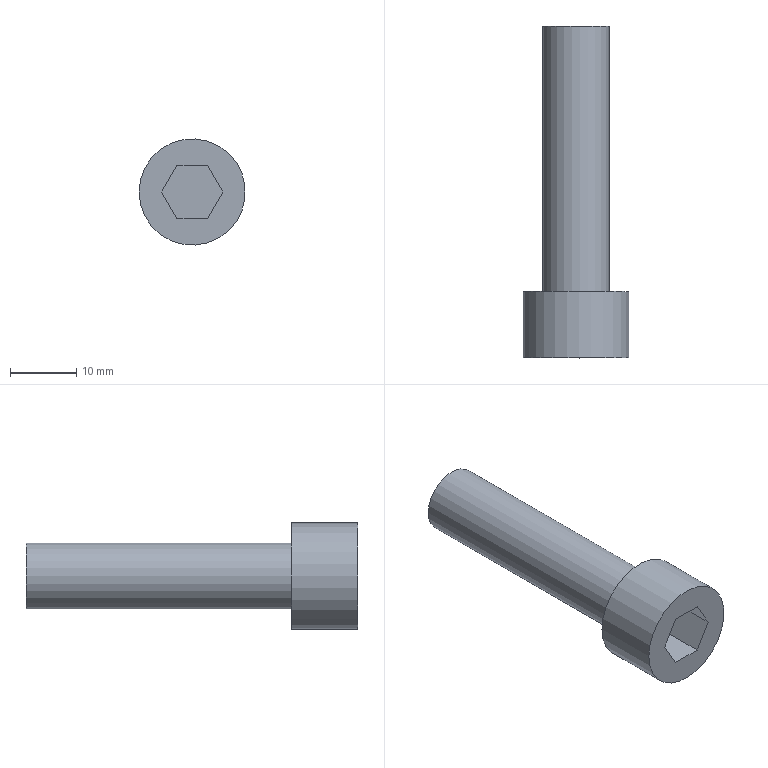Part | STEP file | 1 solid | 12 faces | box 16 x 50 x 16 mm | volume 4786 mm3 | plane 10 | cylinder 2 | commonest cylinder face diameters 10 x1 16 x1
STEP:
#1=CARTESIAN_POINT('',(0.,0.,0.));
#2=DIRECTION('',(0.,0.,1.));
#3=DIRECTION('',(1.,0.,0.));
#4=AXIS2_PLACEMENT_3D('',#1,#2,#3);
#5=CARTESIAN_POINT('',(1368.247,232.48,68.619));
#6=VERTEX_POINT('',#5);
#7=CARTESIAN_POINT('',(1376.247,232.48,68.619));
#8=DIRECTION('',(0.,-1.,0.));
#9=DIRECTION('',(-1.,0.,0.));
#10=AXIS2_PLACEMENT_3D('',#7,#8,#9);
#11=CIRCLE('',#10,8.);
#12=CARTESIAN_POINT('',(1368.247,232.48,68.619));
#13=DIRECTION('',(0.,1.,0.));
#14=DIRECTION('',(1.,0.,0.));
#15=AXIS2_PLACEMENT_3D('',#12,#13,#14);
#16=PLANE('',#15);
#17=CARTESIAN_POINT('',(0.,0.));
#18=CARTESIAN_POINT('',(0.,13.856));
#19=CARTESIAN_POINT('',(12.,6.928));
#20=CARTESIAN_POINT('',(24.,0.));
#21=CARTESIAN_POINT('',(12.,-6.928));
#22=CARTESIAN_POINT('',(0.,-13.856));
#23=CARTESIAN_POINT('',(0.,0.));
#24=(BOUNDED_CURVE()B_SPLINE_CURVE(2,(#17,#18,#19,#20,#21,#22,#23),.UNSPECIFIED.,.T.,.F.)B_SPLINE_CURVE_WITH_KNOTS((1,2,2,2,2,1),(-2.094,0.,2.094,4.189,6.283,8.378),.UNSPECIFIED.)CURVE()GEOMETRIC_REPRESENTATION_ITEM()RATIONAL_B_SPLINE_CURVE((1.,0.5,1.,0.5,1.,0.5,1.))REPRESENTATION_ITEM(''));
#25=(GEOMETRIC_REPRESENTATION_CONTEXT(2)PARAMETRIC_REPRESENTATION_CONTEXT()REPRESENTATION_CONTEXT('',''));
#26=DEFINITIONAL_REPRESENTATION('',(#24),#25);
#27=PCURVE('',#16,#26);
#28=CARTESIAN_POINT('',(1376.247,251.38,68.619));
#29=DIRECTION('',(0.,-1.,0.));
#30=DIRECTION('',(-1.,0.,0.));
#31=AXIS2_PLACEMENT_3D('',#28,#29,#30);
#32=CYLINDRICAL_SURFACE('',#31,8.);
#33=CARTESIAN_POINT('',(0.,18.9));
#34=DIRECTION('',(1.,0.));
#35=VECTOR('',#34,1.);
#36=LINE('',#33,#35);
#37=(GEOMETRIC_REPRESENTATION_CONTEXT(2)PARAMETRIC_REPRESENTATION_CONTEXT()REPRESENTATION_CONTEXT('',''));
#38=DEFINITIONAL_REPRESENTATION('',(#36),#37);
#39=PCURVE('',#32,#38);
#40=SURFACE_CURVE('',#11,(#27,#39),.PCURVE_S1.);
#41=EDGE_CURVE('',#6,#6,#40,.T.);
#42=ORIENTED_EDGE('',*,*,#41,.T.);
#43=EDGE_LOOP('',(#42));
#44=FACE_BOUND('',#43,.T.);
#45=CARTESIAN_POINT('',(1373.938,232.48,72.619));
#46=VERTEX_POINT('',#45);
#47=CARTESIAN_POINT('',(1378.557,232.48,72.619));
#48=VERTEX_POINT('',#47);
#49=CARTESIAN_POINT('',(1378.557,232.48,72.619));
#50=DIRECTION('',(1.,0.,0.));
#51=VECTOR('',#50,1.);
#52=LINE('',#49,#51);
#53=CARTESIAN_POINT('',(10.309,-4.));
#54=DIRECTION('',(1.,0.));
#55=VECTOR('',#54,1.);
#56=LINE('',#53,#55);
#57=(GEOMETRIC_REPRESENTATION_CONTEXT(2)PARAMETRIC_REPRESENTATION_CONTEXT()REPRESENTATION_CONTEXT('',''));
#58=DEFINITIONAL_REPRESENTATION('',(#56),#57);
#59=PCURVE('',#16,#58);
#60=CARTESIAN_POINT('',(1378.557,239.08,72.619));
#61=DIRECTION('',(0.,0.,-1.));
#62=DIRECTION('',(-1.,0.,0.));
#63=AXIS2_PLACEMENT_3D('',#60,#61,#62);
#64=PLANE('',#63);
#65=CARTESIAN_POINT('',(0.,-6.6));
#66=DIRECTION('',(-1.,0.));
#67=VECTOR('',#66,1.);
#68=LINE('',#65,#67);
#69=(GEOMETRIC_REPRESENTATION_CONTEXT(2)PARAMETRIC_REPRESENTATION_CONTEXT()REPRESENTATION_CONTEXT('',''));
#70=DEFINITIONAL_REPRESENTATION('',(#68),#69);
#71=PCURVE('',#64,#70);
#72=SURFACE_CURVE('',#52,(#59,#71),.PCURVE_S1.);
#73=EDGE_CURVE('',#46,#48,#72,.T.);
#74=ORIENTED_EDGE('',*,*,#73,.T.);
#75=CARTESIAN_POINT('',(1380.866,232.48,68.619));
#76=VERTEX_POINT('',#75);
#77=CARTESIAN_POINT('',(1380.866,232.48,68.619));
#78=DIRECTION('',(0.5,0.,-0.866));
#79=VECTOR('',#78,1.);
#80=LINE('',#77,#79);
#81=CARTESIAN_POINT('',(12.619,0.));
#82=DIRECTION('',(0.5,0.866));
#83=VECTOR('',#82,1.);
#84=LINE('',#81,#83);
#85=(GEOMETRIC_REPRESENTATION_CONTEXT(2)PARAMETRIC_REPRESENTATION_CONTEXT()REPRESENTATION_CONTEXT('',''));
#86=DEFINITIONAL_REPRESENTATION('',(#84),#85);
#87=PCURVE('',#16,#86);
#88=CARTESIAN_POINT('',(1380.866,239.08,68.619));
#89=DIRECTION('',(-0.866,0.,-0.5));
#90=DIRECTION('',(-0.5,0.,0.866));
#91=AXIS2_PLACEMENT_3D('',#88,#89,#90);
#92=PLANE('',#91);
#93=CARTESIAN_POINT('',(0.,-6.6));
#94=DIRECTION('',(-1.,0.));
#95=VECTOR('',#94,1.);
#96=LINE('',#93,#95);
#97=(GEOMETRIC_REPRESENTATION_CONTEXT(2)PARAMETRIC_REPRESENTATION_CONTEXT()REPRESENTATION_CONTEXT('',''));
#98=DEFINITIONAL_REPRESENTATION('',(#96),#97);
#99=PCURVE('',#92,#98);
#100=SURFACE_CURVE('',#80,(#87,#99),.PCURVE_S1.);
#101=EDGE_CURVE('',#48,#76,#100,.T.);
#102=ORIENTED_EDGE('',*,*,#101,.T.);
#103=CARTESIAN_POINT('',(1378.557,232.48,64.619));
#104=VERTEX_POINT('',#103);
#105=CARTESIAN_POINT('',(1378.557,232.48,64.619));
#106=DIRECTION('',(-0.5,0.,-0.866));
#107=VECTOR('',#106,1.);
#108=LINE('',#105,#107);
#109=CARTESIAN_POINT('',(10.309,4.));
#110=DIRECTION('',(-0.5,0.866));
#111=VECTOR('',#110,1.);
#112=LINE('',#109,#111);
#113=(GEOMETRIC_REPRESENTATION_CONTEXT(2)PARAMETRIC_REPRESENTATION_CONTEXT()REPRESENTATION_CONTEXT('',''));
#114=DEFINITIONAL_REPRESENTATION('',(#112),#113);
#115=PCURVE('',#16,#114);
#116=CARTESIAN_POINT('',(1378.557,239.08,64.619));
#117=DIRECTION('',(-0.866,0.,0.5));
#118=DIRECTION('',(0.5,0.,0.866));
#119=AXIS2_PLACEMENT_3D('',#116,#117,#118);
#120=PLANE('',#119);
#121=CARTESIAN_POINT('',(0.,-6.6));
#122=DIRECTION('',(-1.,0.));
#123=VECTOR('',#122,1.);
#124=LINE('',#121,#123);
#125=(GEOMETRIC_REPRESENTATION_CONTEXT(2)PARAMETRIC_REPRESENTATION_CONTEXT()REPRESENTATION_CONTEXT('',''));
#126=DEFINITIONAL_REPRESENTATION('',(#124),#125);
#127=PCURVE('',#120,#126);
#128=SURFACE_CURVE('',#108,(#115,#127),.PCURVE_S1.);
#129=EDGE_CURVE('',#76,#104,#128,.T.);
#130=ORIENTED_EDGE('',*,*,#129,.T.);
#131=CARTESIAN_POINT('',(1373.938,232.48,64.619));
#132=VERTEX_POINT('',#131);
#133=CARTESIAN_POINT('',(1373.938,232.48,64.619));
#134=DIRECTION('',(-1.,0.,0.));
#135=VECTOR('',#134,1.);
#136=LINE('',#133,#135);
#137=CARTESIAN_POINT('',(5.691,4.));
#138=DIRECTION('',(-1.,0.));
#139=VECTOR('',#138,1.);
#140=LINE('',#137,#139);
#141=(GEOMETRIC_REPRESENTATION_CONTEXT(2)PARAMETRIC_REPRESENTATION_CONTEXT()REPRESENTATION_CONTEXT('',''));
#142=DEFINITIONAL_REPRESENTATION('',(#140),#141);
#143=PCURVE('',#16,#142);
#144=CARTESIAN_POINT('',(1373.938,239.08,64.619));
#145=DIRECTION('',(0.,0.,1.));
#146=DIRECTION('',(1.,0.,0.));
#147=AXIS2_PLACEMENT_3D('',#144,#145,#146);
#148=PLANE('',#147);
#149=CARTESIAN_POINT('',(0.,-6.6));
#150=DIRECTION('',(-1.,0.));
#151=VECTOR('',#150,1.);
#152=LINE('',#149,#151);
#153=(GEOMETRIC_REPRESENTATION_CONTEXT(2)PARAMETRIC_REPRESENTATION_CONTEXT()REPRESENTATION_CONTEXT('',''));
#154=DEFINITIONAL_REPRESENTATION('',(#152),#153);
#155=PCURVE('',#148,#154);
#156=SURFACE_CURVE('',#136,(#143,#155),.PCURVE_S1.);
#157=EDGE_CURVE('',#104,#132,#156,.T.);
#158=ORIENTED_EDGE('',*,*,#157,.T.);
#159=CARTESIAN_POINT('',(1371.628,232.48,68.619));
#160=VERTEX_POINT('',#159);
#161=CARTESIAN_POINT('',(1371.628,232.48,68.619));
#162=DIRECTION('',(-0.5,0.,0.866));
#163=VECTOR('',#162,1.);
#164=LINE('',#161,#163);
#165=CARTESIAN_POINT('',(3.381,0.));
#166=DIRECTION('',(-0.5,-0.866));
#167=VECTOR('',#166,1.);
#168=LINE('',#165,#167);
#169=(GEOMETRIC_REPRESENTATION_CONTEXT(2)PARAMETRIC_REPRESENTATION_CONTEXT()REPRESENTATION_CONTEXT('',''));
#170=DEFINITIONAL_REPRESENTATION('',(#168),#169);
#171=PCURVE('',#16,#170);
#172=CARTESIAN_POINT('',(1371.628,239.08,68.619));
#173=DIRECTION('',(0.866,0.,0.5));
#174=DIRECTION('',(0.5,0.,-0.866));
#175=AXIS2_PLACEMENT_3D('',#172,#173,#174);
#176=PLANE('',#175);
#177=CARTESIAN_POINT('',(0.,-6.6));
#178=DIRECTION('',(-1.,0.));
#179=VECTOR('',#178,1.);
#180=LINE('',#177,#179);
#181=(GEOMETRIC_REPRESENTATION_CONTEXT(2)PARAMETRIC_REPRESENTATION_CONTEXT()REPRESENTATION_CONTEXT('',''));
#182=DEFINITIONAL_REPRESENTATION('',(#180),#181);
#183=PCURVE('',#176,#182);
#184=SURFACE_CURVE('',#164,(#171,#183),.PCURVE_S1.);
#185=EDGE_CURVE('',#132,#160,#184,.T.);
#186=ORIENTED_EDGE('',*,*,#185,.T.);
#187=CARTESIAN_POINT('',(1373.938,232.48,72.619));
#188=DIRECTION('',(0.5,0.,0.866));
#189=VECTOR('',#188,1.);
#190=LINE('',#187,#189);
#191=CARTESIAN_POINT('',(5.691,-4.));
#192=DIRECTION('',(0.5,-0.866));
#193=VECTOR('',#192,1.);
#194=LINE('',#191,#193);
#195=(GEOMETRIC_REPRESENTATION_CONTEXT(2)PARAMETRIC_REPRESENTATION_CONTEXT()REPRESENTATION_CONTEXT('',''));
#196=DEFINITIONAL_REPRESENTATION('',(#194),#195);
#197=PCURVE('',#16,#196);
#198=CARTESIAN_POINT('',(1373.938,239.08,72.619));
#199=DIRECTION('',(0.866,0.,-0.5));
#200=DIRECTION('',(-0.5,0.,-0.866));
#201=AXIS2_PLACEMENT_3D('',#198,#199,#200);
#202=PLANE('',#201);
#203=CARTESIAN_POINT('',(0.,-6.6));
#204=DIRECTION('',(-1.,0.));
#205=VECTOR('',#204,1.);
#206=LINE('',#203,#205);
#207=(GEOMETRIC_REPRESENTATION_CONTEXT(2)PARAMETRIC_REPRESENTATION_CONTEXT()REPRESENTATION_CONTEXT('',''));
#208=DEFINITIONAL_REPRESENTATION('',(#206),#207);
#209=PCURVE('',#202,#208);
#210=SURFACE_CURVE('',#190,(#197,#209),.PCURVE_S1.);
#211=EDGE_CURVE('',#160,#46,#210,.T.);
#212=ORIENTED_EDGE('',*,*,#211,.T.);
#213=EDGE_LOOP('',(#74,#102,#130,#158,#186,#212));
#214=FACE_BOUND('',#213,.T.);
#215=ADVANCED_FACE('',(#44,#214),#16,.F.);
#216=ORIENTED_EDGE('',*,*,#41,.F.);
#217=CARTESIAN_POINT('',(1368.247,242.48,68.619));
#218=VERTEX_POINT('',#217);
#219=CARTESIAN_POINT('',(1368.247,242.48,68.619));
#220=CARTESIAN_POINT('',(1368.247,232.48,68.619));
#221=B_SPLINE_CURVE_WITH_KNOTS('',1,(#219,#220),.UNSPECIFIED.,.F.,.F.,(2,2),(8.9,18.9),.PIECEWISE_BEZIER_KNOTS.);
#222=CARTESIAN_POINT('',(0.,0.));
#223=DIRECTION('',(0.,1.));
#224=VECTOR('',#223,1.);
#225=LINE('',#222,#224);
#226=(GEOMETRIC_REPRESENTATION_CONTEXT(2)PARAMETRIC_REPRESENTATION_CONTEXT()REPRESENTATION_CONTEXT('',''));
#227=DEFINITIONAL_REPRESENTATION('',(#225),#226);
#228=PCURVE('',#32,#227);
#229=CARTESIAN_POINT('',(6.283,0.));
#230=DIRECTION('',(0.,1.));
#231=VECTOR('',#230,1.);
#232=LINE('',#229,#231);
#233=(GEOMETRIC_REPRESENTATION_CONTEXT(2)PARAMETRIC_REPRESENTATION_CONTEXT()REPRESENTATION_CONTEXT('',''));
#234=DEFINITIONAL_REPRESENTATION('',(#232),#233);
#235=PCURVE('',#32,#234);
#236=SEAM_CURVE('',#221,(#228,#235),.PCURVE_S1.);
#237=EDGE_CURVE('',#218,#6,#236,.T.);
#238=ORIENTED_EDGE('',*,*,#237,.F.);
#239=CARTESIAN_POINT('',(1376.247,242.48,68.619));
#240=DIRECTION('',(0.,-1.,0.));
#241=DIRECTION('',(-1.,0.,0.));
#242=AXIS2_PLACEMENT_3D('',#239,#240,#241);
#243=CIRCLE('',#242,8.);
#244=CARTESIAN_POINT('',(0.,8.9));
#245=DIRECTION('',(1.,0.));
#246=VECTOR('',#245,1.);
#247=LINE('',#244,#246);
#248=(GEOMETRIC_REPRESENTATION_CONTEXT(2)PARAMETRIC_REPRESENTATION_CONTEXT()REPRESENTATION_CONTEXT('',''));
#249=DEFINITIONAL_REPRESENTATION('',(#247),#248);
#250=PCURVE('',#32,#249);
#251=CARTESIAN_POINT('',(1371.247,242.48,68.619));
#252=DIRECTION('',(0.,-1.,0.));
#253=DIRECTION('',(-1.,0.,0.));
#254=AXIS2_PLACEMENT_3D('',#251,#252,#253);
#255=PLANE('',#254);
#256=CARTESIAN_POINT('',(-5.,0.));
#257=DIRECTION('',(1.,0.));
#258=AXIS2_PLACEMENT_2D('',#256,#257);
#259=CIRCLE('',#258,8.);
#260=(GEOMETRIC_REPRESENTATION_CONTEXT(2)PARAMETRIC_REPRESENTATION_CONTEXT()REPRESENTATION_CONTEXT('',''));
#261=DEFINITIONAL_REPRESENTATION('',(#259),#260);
#262=PCURVE('',#255,#261);
#263=SURFACE_CURVE('',#243,(#250,#262),.PCURVE_S1.);
#264=EDGE_CURVE('',#218,#218,#263,.T.);
#265=ORIENTED_EDGE('',*,*,#264,.T.);
#266=ORIENTED_EDGE('',*,*,#237,.T.);
#267=EDGE_LOOP('',(#216,#238,#265,#266));
#268=FACE_BOUND('',#267,.T.);
#269=ADVANCED_FACE('',(#268),#32,.T.);
#270=ORIENTED_EDGE('',*,*,#264,.F.);
#271=EDGE_LOOP('',(#270));
#272=FACE_BOUND('',#271,.T.);
#273=CARTESIAN_POINT('',(1371.247,242.48,68.619));
#274=VERTEX_POINT('',#273);
#275=CARTESIAN_POINT('',(1376.247,242.48,68.619));
#276=DIRECTION('',(0.,-1.,0.));
#277=DIRECTION('',(-1.,0.,0.));
#278=AXIS2_PLACEMENT_3D('',#275,#276,#277);
#279=CIRCLE('',#278,5.);
#280=CARTESIAN_POINT('',(-5.,0.));
#281=DIRECTION('',(1.,0.));
#282=AXIS2_PLACEMENT_2D('',#280,#281);
#283=CIRCLE('',#282,5.);
#284=(GEOMETRIC_REPRESENTATION_CONTEXT(2)PARAMETRIC_REPRESENTATION_CONTEXT()REPRESENTATION_CONTEXT('',''));
#285=DEFINITIONAL_REPRESENTATION('',(#283),#284);
#286=PCURVE('',#255,#285);
#287=CARTESIAN_POINT('',(1376.247,251.38,68.619));
#288=DIRECTION('',(0.,-1.,0.));
#289=DIRECTION('',(-1.,0.,0.));
#290=AXIS2_PLACEMENT_3D('',#287,#288,#289);
#291=CYLINDRICAL_SURFACE('',#290,5.);
#292=CARTESIAN_POINT('',(0.,8.9));
#293=DIRECTION('',(1.,0.));
#294=VECTOR('',#293,1.);
#295=LINE('',#292,#294);
#296=(GEOMETRIC_REPRESENTATION_CONTEXT(2)PARAMETRIC_REPRESENTATION_CONTEXT()REPRESENTATION_CONTEXT('',''));
#297=DEFINITIONAL_REPRESENTATION('',(#295),#296);
#298=PCURVE('',#291,#297);
#299=SURFACE_CURVE('',#279,(#286,#298),.PCURVE_S1.);
#300=EDGE_CURVE('',#274,#274,#299,.T.);
#301=ORIENTED_EDGE('',*,*,#300,.T.);
#302=EDGE_LOOP('',(#301));
#303=FACE_BOUND('',#302,.T.);
#304=ADVANCED_FACE('',(#272,#303),#255,.F.);
#305=ORIENTED_EDGE('',*,*,#300,.F.);
#306=CARTESIAN_POINT('',(1371.247,282.48,68.619));
#307=VERTEX_POINT('',#306);
#308=CARTESIAN_POINT('',(1371.247,282.48,68.619));
#309=CARTESIAN_POINT('',(1371.247,242.48,68.619));
#310=B_SPLINE_CURVE_WITH_KNOTS('',1,(#308,#309),.UNSPECIFIED.,.F.,.F.,(2,2),(-31.1,8.9),.PIECEWISE_BEZIER_KNOTS.);
#311=CARTESIAN_POINT('',(0.,0.));
#312=DIRECTION('',(0.,1.));
#313=VECTOR('',#312,1.);
#314=LINE('',#311,#313);
#315=(GEOMETRIC_REPRESENTATION_CONTEXT(2)PARAMETRIC_REPRESENTATION_CONTEXT()REPRESENTATION_CONTEXT('',''));
#316=DEFINITIONAL_REPRESENTATION('',(#314),#315);
#317=PCURVE('',#291,#316);
#318=CARTESIAN_POINT('',(6.283,0.));
#319=DIRECTION('',(0.,1.));
#320=VECTOR('',#319,1.);
#321=LINE('',#318,#320);
#322=(GEOMETRIC_REPRESENTATION_CONTEXT(2)PARAMETRIC_REPRESENTATION_CONTEXT()REPRESENTATION_CONTEXT('',''));
#323=DEFINITIONAL_REPRESENTATION('',(#321),#322);
#324=PCURVE('',#291,#323);
#325=SEAM_CURVE('',#310,(#317,#324),.PCURVE_S1.);
#326=EDGE_CURVE('',#307,#274,#325,.T.);
#327=ORIENTED_EDGE('',*,*,#326,.F.);
#328=CARTESIAN_POINT('',(1376.247,282.48,68.619));
#329=DIRECTION('',(0.,-1.,0.));
#330=DIRECTION('',(-1.,0.,0.));
#331=AXIS2_PLACEMENT_3D('',#328,#329,#330);
#332=CIRCLE('',#331,5.);
#333=CARTESIAN_POINT('',(0.,-31.1));
#334=DIRECTION('',(1.,0.));
#335=VECTOR('',#334,1.);
#336=LINE('',#333,#335);
#337=(GEOMETRIC_REPRESENTATION_CONTEXT(2)PARAMETRIC_REPRESENTATION_CONTEXT()REPRESENTATION_CONTEXT('',''));
#338=DEFINITIONAL_REPRESENTATION('',(#336),#337);
#339=PCURVE('',#291,#338);
#340=CARTESIAN_POINT('',(1376.247,282.48,68.619));
#341=DIRECTION('',(0.,-1.,0.));
#342=DIRECTION('',(-1.,0.,0.));
#343=AXIS2_PLACEMENT_3D('',#340,#341,#342);
#344=PLANE('',#343);
#345=CARTESIAN_POINT('',(0.,0.));
#346=DIRECTION('',(1.,0.));
#347=AXIS2_PLACEMENT_2D('',#345,#346);
#348=CIRCLE('',#347,5.);
#349=(GEOMETRIC_REPRESENTATION_CONTEXT(2)PARAMETRIC_REPRESENTATION_CONTEXT()REPRESENTATION_CONTEXT('',''));
#350=DEFINITIONAL_REPRESENTATION('',(#348),#349);
#351=PCURVE('',#344,#350);
#352=SURFACE_CURVE('',#332,(#339,#351),.PCURVE_S1.);
#353=EDGE_CURVE('',#307,#307,#352,.T.);
#354=ORIENTED_EDGE('',*,*,#353,.T.);
#355=ORIENTED_EDGE('',*,*,#326,.T.);
#356=EDGE_LOOP('',(#305,#327,#354,#355));
#357=FACE_BOUND('',#356,.T.);
#358=ADVANCED_FACE('',(#357),#291,.T.);
#359=ORIENTED_EDGE('',*,*,#353,.F.);
#360=EDGE_LOOP('',(#359));
#361=FACE_BOUND('',#360,.T.);
#362=ADVANCED_FACE('',(#361),#344,.F.);
#363=ORIENTED_EDGE('',*,*,#73,.F.);
#364=CARTESIAN_POINT('',(1373.938,239.08,72.619));
#365=VERTEX_POINT('',#364);
#366=CARTESIAN_POINT('',(1373.938,239.08,72.619));
#367=DIRECTION('',(0.,-1.,0.));
#368=VECTOR('',#367,1.);
#369=LINE('',#366,#368);
#370=CARTESIAN_POINT('',(4.619,0.));
#371=DIRECTION('',(0.,-1.));
#372=VECTOR('',#371,1.);
#373=LINE('',#370,#372);
#374=(GEOMETRIC_REPRESENTATION_CONTEXT(2)PARAMETRIC_REPRESENTATION_CONTEXT()REPRESENTATION_CONTEXT('',''));
#375=DEFINITIONAL_REPRESENTATION('',(#373),#374);
#376=PCURVE('',#64,#375);
#377=CARTESIAN_POINT('',(0.,0.));
#378=DIRECTION('',(0.,-1.));
#379=VECTOR('',#378,1.);
#380=LINE('',#377,#379);
#381=(GEOMETRIC_REPRESENTATION_CONTEXT(2)PARAMETRIC_REPRESENTATION_CONTEXT()REPRESENTATION_CONTEXT('',''));
#382=DEFINITIONAL_REPRESENTATION('',(#380),#381);
#383=PCURVE('',#202,#382);
#384=SURFACE_CURVE('',#369,(#376,#383),.PCURVE_S1.);
#385=EDGE_CURVE('',#365,#46,#384,.T.);
#386=ORIENTED_EDGE('',*,*,#385,.F.);
#387=CARTESIAN_POINT('',(1378.557,239.08,72.619));
#388=VERTEX_POINT('',#387);
#389=CARTESIAN_POINT('',(1378.557,239.08,72.619));
#390=DIRECTION('',(-1.,0.,0.));
#391=VECTOR('',#390,1.);
#392=LINE('',#389,#391);
#393=CARTESIAN_POINT('',(0.,0.));
#394=DIRECTION('',(1.,0.));
#395=VECTOR('',#394,1.);
#396=LINE('',#393,#395);
#397=(GEOMETRIC_REPRESENTATION_CONTEXT(2)PARAMETRIC_REPRESENTATION_CONTEXT()REPRESENTATION_CONTEXT('',''));
#398=DEFINITIONAL_REPRESENTATION('',(#396),#397);
#399=PCURVE('',#64,#398);
#400=CARTESIAN_POINT('',(1376.247,239.08,68.619));
#401=DIRECTION('',(0.,1.,0.));
#402=DIRECTION('',(1.,0.,0.));
#403=AXIS2_PLACEMENT_3D('',#400,#401,#402);
#404=PLANE('',#403);
#405=CARTESIAN_POINT('',(2.309,-4.));
#406=DIRECTION('',(-1.,0.));
#407=VECTOR('',#406,1.);
#408=LINE('',#405,#407);
#409=(GEOMETRIC_REPRESENTATION_CONTEXT(2)PARAMETRIC_REPRESENTATION_CONTEXT()REPRESENTATION_CONTEXT('',''));
#410=DEFINITIONAL_REPRESENTATION('',(#408),#409);
#411=PCURVE('',#404,#410);
#412=SURFACE_CURVE('',#392,(#399,#411),.PCURVE_S1.);
#413=EDGE_CURVE('',#388,#365,#412,.T.);
#414=ORIENTED_EDGE('',*,*,#413,.F.);
#415=CARTESIAN_POINT('',(1378.557,239.08,72.619));
#416=DIRECTION('',(0.,-1.,0.));
#417=VECTOR('',#416,1.);
#418=LINE('',#415,#417);
#419=CARTESIAN_POINT('',(0.,0.));
#420=DIRECTION('',(0.,-1.));
#421=VECTOR('',#420,1.);
#422=LINE('',#419,#421);
#423=(GEOMETRIC_REPRESENTATION_CONTEXT(2)PARAMETRIC_REPRESENTATION_CONTEXT()REPRESENTATION_CONTEXT('',''));
#424=DEFINITIONAL_REPRESENTATION('',(#422),#423);
#425=PCURVE('',#64,#424);
#426=CARTESIAN_POINT('',(4.619,0.));
#427=DIRECTION('',(0.,-1.));
#428=VECTOR('',#427,1.);
#429=LINE('',#426,#428);
#430=(GEOMETRIC_REPRESENTATION_CONTEXT(2)PARAMETRIC_REPRESENTATION_CONTEXT()REPRESENTATION_CONTEXT('',''));
#431=DEFINITIONAL_REPRESENTATION('',(#429),#430);
#432=PCURVE('',#92,#431);
#433=SURFACE_CURVE('',#418,(#425,#432),.PCURVE_S1.);
#434=EDGE_CURVE('',#388,#48,#433,.T.);
#435=ORIENTED_EDGE('',*,*,#434,.T.);
#436=EDGE_LOOP('',(#363,#386,#414,#435));
#437=FACE_BOUND('',#436,.T.);
#438=ADVANCED_FACE('',(#437),#64,.T.);
#439=ORIENTED_EDGE('',*,*,#211,.F.);
#440=CARTESIAN_POINT('',(1371.628,239.08,68.619));
#441=VERTEX_POINT('',#440);
#442=CARTESIAN_POINT('',(1371.628,239.08,68.619));
#443=DIRECTION('',(0.,-1.,0.));
#444=VECTOR('',#443,1.);
#445=LINE('',#442,#444);
#446=CARTESIAN_POINT('',(4.619,0.));
#447=DIRECTION('',(0.,-1.));
#448=VECTOR('',#447,1.);
#449=LINE('',#446,#448);
#450=(GEOMETRIC_REPRESENTATION_CONTEXT(2)PARAMETRIC_REPRESENTATION_CONTEXT()REPRESENTATION_CONTEXT('',''));
#451=DEFINITIONAL_REPRESENTATION('',(#449),#450);
#452=PCURVE('',#202,#451);
#453=CARTESIAN_POINT('',(0.,0.));
#454=DIRECTION('',(0.,-1.));
#455=VECTOR('',#454,1.);
#456=LINE('',#453,#455);
#457=(GEOMETRIC_REPRESENTATION_CONTEXT(2)PARAMETRIC_REPRESENTATION_CONTEXT()REPRESENTATION_CONTEXT('',''));
#458=DEFINITIONAL_REPRESENTATION('',(#456),#457);
#459=PCURVE('',#176,#458);
#460=SURFACE_CURVE('',#445,(#452,#459),.PCURVE_S1.);
#461=EDGE_CURVE('',#441,#160,#460,.T.);
#462=ORIENTED_EDGE('',*,*,#461,.F.);
#463=CARTESIAN_POINT('',(1373.938,239.08,72.619));
#464=DIRECTION('',(-0.5,0.,-0.866));
#465=VECTOR('',#464,1.);
#466=LINE('',#463,#465);
#467=CARTESIAN_POINT('',(0.,0.));
#468=DIRECTION('',(1.,0.));
#469=VECTOR('',#468,1.);
#470=LINE('',#467,#469);
#471=(GEOMETRIC_REPRESENTATION_CONTEXT(2)PARAMETRIC_REPRESENTATION_CONTEXT()REPRESENTATION_CONTEXT('',''));
#472=DEFINITIONAL_REPRESENTATION('',(#470),#471);
#473=PCURVE('',#202,#472);
#474=CARTESIAN_POINT('',(-2.309,-4.));
#475=DIRECTION('',(-0.5,0.866));
#476=VECTOR('',#475,1.);
#477=LINE('',#474,#476);
#478=(GEOMETRIC_REPRESENTATION_CONTEXT(2)PARAMETRIC_REPRESENTATION_CONTEXT()REPRESENTATION_CONTEXT('',''));
#479=DEFINITIONAL_REPRESENTATION('',(#477),#478);
#480=PCURVE('',#404,#479);
#481=SURFACE_CURVE('',#466,(#473,#480),.PCURVE_S1.);
#482=EDGE_CURVE('',#365,#441,#481,.T.);
#483=ORIENTED_EDGE('',*,*,#482,.F.);
#484=ORIENTED_EDGE('',*,*,#385,.T.);
#485=EDGE_LOOP('',(#439,#462,#483,#484));
#486=FACE_BOUND('',#485,.T.);
#487=ADVANCED_FACE('',(#486),#202,.T.);
#488=ORIENTED_EDGE('',*,*,#185,.F.);
#489=CARTESIAN_POINT('',(1373.938,239.08,64.619));
#490=VERTEX_POINT('',#489);
#491=CARTESIAN_POINT('',(1373.938,239.08,64.619));
#492=DIRECTION('',(0.,-1.,0.));
#493=VECTOR('',#492,1.);
#494=LINE('',#491,#493);
#495=CARTESIAN_POINT('',(4.619,0.));
#496=DIRECTION('',(0.,-1.));
#497=VECTOR('',#496,1.);
#498=LINE('',#495,#497);
#499=(GEOMETRIC_REPRESENTATION_CONTEXT(2)PARAMETRIC_REPRESENTATION_CONTEXT()REPRESENTATION_CONTEXT('',''));
#500=DEFINITIONAL_REPRESENTATION('',(#498),#499);
#501=PCURVE('',#176,#500);
#502=CARTESIAN_POINT('',(0.,0.));
#503=DIRECTION('',(0.,-1.));
#504=VECTOR('',#503,1.);
#505=LINE('',#502,#504);
#506=(GEOMETRIC_REPRESENTATION_CONTEXT(2)PARAMETRIC_REPRESENTATION_CONTEXT()REPRESENTATION_CONTEXT('',''));
#507=DEFINITIONAL_REPRESENTATION('',(#505),#506);
#508=PCURVE('',#148,#507);
#509=SURFACE_CURVE('',#494,(#501,#508),.PCURVE_S1.);
#510=EDGE_CURVE('',#490,#132,#509,.T.);
#511=ORIENTED_EDGE('',*,*,#510,.F.);
#512=CARTESIAN_POINT('',(1371.628,239.08,68.619));
#513=DIRECTION('',(0.5,0.,-0.866));
#514=VECTOR('',#513,1.);
#515=LINE('',#512,#514);
#516=CARTESIAN_POINT('',(0.,0.));
#517=DIRECTION('',(1.,0.));
#518=VECTOR('',#517,1.);
#519=LINE('',#516,#518);
#520=(GEOMETRIC_REPRESENTATION_CONTEXT(2)PARAMETRIC_REPRESENTATION_CONTEXT()REPRESENTATION_CONTEXT('',''));
#521=DEFINITIONAL_REPRESENTATION('',(#519),#520);
#522=PCURVE('',#176,#521);
#523=CARTESIAN_POINT('',(-4.619,0.));
#524=DIRECTION('',(0.5,0.866));
#525=VECTOR('',#524,1.);
#526=LINE('',#523,#525);
#527=(GEOMETRIC_REPRESENTATION_CONTEXT(2)PARAMETRIC_REPRESENTATION_CONTEXT()REPRESENTATION_CONTEXT('',''));
#528=DEFINITIONAL_REPRESENTATION('',(#526),#527);
#529=PCURVE('',#404,#528);
#530=SURFACE_CURVE('',#515,(#522,#529),.PCURVE_S1.);
#531=EDGE_CURVE('',#441,#490,#530,.T.);
#532=ORIENTED_EDGE('',*,*,#531,.F.);
#533=ORIENTED_EDGE('',*,*,#461,.T.);
#534=EDGE_LOOP('',(#488,#511,#532,#533));
#535=FACE_BOUND('',#534,.T.);
#536=ADVANCED_FACE('',(#535),#176,.T.);
#537=ORIENTED_EDGE('',*,*,#157,.F.);
#538=CARTESIAN_POINT('',(1378.557,239.08,64.619));
#539=VERTEX_POINT('',#538);
#540=CARTESIAN_POINT('',(1378.557,239.08,64.619));
#541=DIRECTION('',(0.,-1.,0.));
#542=VECTOR('',#541,1.);
#543=LINE('',#540,#542);
#544=CARTESIAN_POINT('',(4.619,0.));
#545=DIRECTION('',(0.,-1.));
#546=VECTOR('',#545,1.);
#547=LINE('',#544,#546);
#548=(GEOMETRIC_REPRESENTATION_CONTEXT(2)PARAMETRIC_REPRESENTATION_CONTEXT()REPRESENTATION_CONTEXT('',''));
#549=DEFINITIONAL_REPRESENTATION('',(#547),#548);
#550=PCURVE('',#148,#549);
#551=CARTESIAN_POINT('',(0.,0.));
#552=DIRECTION('',(0.,-1.));
#553=VECTOR('',#552,1.);
#554=LINE('',#551,#553);
#555=(GEOMETRIC_REPRESENTATION_CONTEXT(2)PARAMETRIC_REPRESENTATION_CONTEXT()REPRESENTATION_CONTEXT('',''));
#556=DEFINITIONAL_REPRESENTATION('',(#554),#555);
#557=PCURVE('',#120,#556);
#558=SURFACE_CURVE('',#543,(#550,#557),.PCURVE_S1.);
#559=EDGE_CURVE('',#539,#104,#558,.T.);
#560=ORIENTED_EDGE('',*,*,#559,.F.);
#561=CARTESIAN_POINT('',(1373.938,239.08,64.619));
#562=DIRECTION('',(1.,0.,0.));
#563=VECTOR('',#562,1.);
#564=LINE('',#561,#563);
#565=CARTESIAN_POINT('',(0.,0.));
#566=DIRECTION('',(1.,0.));
#567=VECTOR('',#566,1.);
#568=LINE('',#565,#567);
#569=(GEOMETRIC_REPRESENTATION_CONTEXT(2)PARAMETRIC_REPRESENTATION_CONTEXT()REPRESENTATION_CONTEXT('',''));
#570=DEFINITIONAL_REPRESENTATION('',(#568),#569);
#571=PCURVE('',#148,#570);
#572=CARTESIAN_POINT('',(-2.309,4.));
#573=DIRECTION('',(1.,0.));
#574=VECTOR('',#573,1.);
#575=LINE('',#572,#574);
#576=(GEOMETRIC_REPRESENTATION_CONTEXT(2)PARAMETRIC_REPRESENTATION_CONTEXT()REPRESENTATION_CONTEXT('',''));
#577=DEFINITIONAL_REPRESENTATION('',(#575),#576);
#578=PCURVE('',#404,#577);
#579=SURFACE_CURVE('',#564,(#571,#578),.PCURVE_S1.);
#580=EDGE_CURVE('',#490,#539,#579,.T.);
#581=ORIENTED_EDGE('',*,*,#580,.F.);
#582=ORIENTED_EDGE('',*,*,#510,.T.);
#583=EDGE_LOOP('',(#537,#560,#581,#582));
#584=FACE_BOUND('',#583,.T.);
#585=ADVANCED_FACE('',(#584),#148,.T.);
#586=ORIENTED_EDGE('',*,*,#129,.F.);
#587=CARTESIAN_POINT('',(1380.866,239.08,68.619));
#588=VERTEX_POINT('',#587);
#589=CARTESIAN_POINT('',(1380.866,239.08,68.619));
#590=DIRECTION('',(0.,-1.,0.));
#591=VECTOR('',#590,1.);
#592=LINE('',#589,#591);
#593=CARTESIAN_POINT('',(4.619,0.));
#594=DIRECTION('',(0.,-1.));
#595=VECTOR('',#594,1.);
#596=LINE('',#593,#595);
#597=(GEOMETRIC_REPRESENTATION_CONTEXT(2)PARAMETRIC_REPRESENTATION_CONTEXT()REPRESENTATION_CONTEXT('',''));
#598=DEFINITIONAL_REPRESENTATION('',(#596),#597);
#599=PCURVE('',#120,#598);
#600=CARTESIAN_POINT('',(0.,0.));
#601=DIRECTION('',(0.,-1.));
#602=VECTOR('',#601,1.);
#603=LINE('',#600,#602);
#604=(GEOMETRIC_REPRESENTATION_CONTEXT(2)PARAMETRIC_REPRESENTATION_CONTEXT()REPRESENTATION_CONTEXT('',''));
#605=DEFINITIONAL_REPRESENTATION('',(#603),#604);
#606=PCURVE('',#92,#605);
#607=SURFACE_CURVE('',#592,(#599,#606),.PCURVE_S1.);
#608=EDGE_CURVE('',#588,#76,#607,.T.);
#609=ORIENTED_EDGE('',*,*,#608,.F.);
#610=CARTESIAN_POINT('',(1378.557,239.08,64.619));
#611=DIRECTION('',(0.5,0.,0.866));
#612=VECTOR('',#611,1.);
#613=LINE('',#610,#612);
#614=CARTESIAN_POINT('',(0.,0.));
#615=DIRECTION('',(1.,0.));
#616=VECTOR('',#615,1.);
#617=LINE('',#614,#616);
#618=(GEOMETRIC_REPRESENTATION_CONTEXT(2)PARAMETRIC_REPRESENTATION_CONTEXT()REPRESENTATION_CONTEXT('',''));
#619=DEFINITIONAL_REPRESENTATION('',(#617),#618);
#620=PCURVE('',#120,#619);
#621=CARTESIAN_POINT('',(2.309,4.));
#622=DIRECTION('',(0.5,-0.866));
#623=VECTOR('',#622,1.);
#624=LINE('',#621,#623);
#625=(GEOMETRIC_REPRESENTATION_CONTEXT(2)PARAMETRIC_REPRESENTATION_CONTEXT()REPRESENTATION_CONTEXT('',''));
#626=DEFINITIONAL_REPRESENTATION('',(#624),#625);
#627=PCURVE('',#404,#626);
#628=SURFACE_CURVE('',#613,(#620,#627),.PCURVE_S1.);
#629=EDGE_CURVE('',#539,#588,#628,.T.);
#630=ORIENTED_EDGE('',*,*,#629,.F.);
#631=ORIENTED_EDGE('',*,*,#559,.T.);
#632=EDGE_LOOP('',(#586,#609,#630,#631));
#633=FACE_BOUND('',#632,.T.);
#634=ADVANCED_FACE('',(#633),#120,.T.);
#635=ORIENTED_EDGE('',*,*,#101,.F.);
#636=ORIENTED_EDGE('',*,*,#434,.F.);
#637=CARTESIAN_POINT('',(1380.866,239.08,68.619));
#638=DIRECTION('',(-0.5,0.,0.866));
#639=VECTOR('',#638,1.);
#640=LINE('',#637,#639);
#641=CARTESIAN_POINT('',(0.,0.));
#642=DIRECTION('',(1.,0.));
#643=VECTOR('',#642,1.);
#644=LINE('',#641,#643);
#645=(GEOMETRIC_REPRESENTATION_CONTEXT(2)PARAMETRIC_REPRESENTATION_CONTEXT()REPRESENTATION_CONTEXT('',''));
#646=DEFINITIONAL_REPRESENTATION('',(#644),#645);
#647=PCURVE('',#92,#646);
#648=CARTESIAN_POINT('',(4.619,0.));
#649=DIRECTION('',(-0.5,-0.866));
#650=VECTOR('',#649,1.);
#651=LINE('',#648,#650);
#652=(GEOMETRIC_REPRESENTATION_CONTEXT(2)PARAMETRIC_REPRESENTATION_CONTEXT()REPRESENTATION_CONTEXT('',''));
#653=DEFINITIONAL_REPRESENTATION('',(#651),#652);
#654=PCURVE('',#404,#653);
#655=SURFACE_CURVE('',#640,(#647,#654),.PCURVE_S1.);
#656=EDGE_CURVE('',#588,#388,#655,.T.);
#657=ORIENTED_EDGE('',*,*,#656,.F.);
#658=ORIENTED_EDGE('',*,*,#608,.T.);
#659=EDGE_LOOP('',(#635,#636,#657,#658));
#660=FACE_BOUND('',#659,.T.);
#661=ADVANCED_FACE('',(#660),#92,.T.);
#662=ORIENTED_EDGE('',*,*,#413,.T.);
#663=ORIENTED_EDGE('',*,*,#482,.T.);
#664=ORIENTED_EDGE('',*,*,#531,.T.);
#665=ORIENTED_EDGE('',*,*,#580,.T.);
#666=ORIENTED_EDGE('',*,*,#629,.T.);
#667=ORIENTED_EDGE('',*,*,#656,.T.);
#668=EDGE_LOOP('',(#662,#663,#664,#665,#666,#667));
#669=FACE_BOUND('',#668,.T.);
#670=ADVANCED_FACE('',(#669),#404,.F.);
#671=CLOSED_SHELL('',(#215,#269,#304,#358,#362,#438,#487,#536,#585,#634,#661,#670));
#672=MANIFOLD_SOLID_BREP('',#671);
#673=(LENGTH_UNIT()NAMED_UNIT(*)SI_UNIT(.MILLI.,.METRE.));
#674=UNCERTAINTY_MEASURE_WITH_UNIT(LENGTH_MEASURE(0.000002),#673,'','');
#675=(NAMED_UNIT(*)PLANE_ANGLE_UNIT()SI_UNIT($,.RADIAN.));
#676=(NAMED_UNIT(*)SI_UNIT($,.STERADIAN.)SOLID_ANGLE_UNIT());
#677=(GEOMETRIC_REPRESENTATION_CONTEXT(3)GLOBAL_UNCERTAINTY_ASSIGNED_CONTEXT((#674))GLOBAL_UNIT_ASSIGNED_CONTEXT((#673,#675,#676))REPRESENTATION_CONTEXT('',''));
#678=ADVANCED_BREP_SHAPE_REPRESENTATION('',(#4,#672),#677);